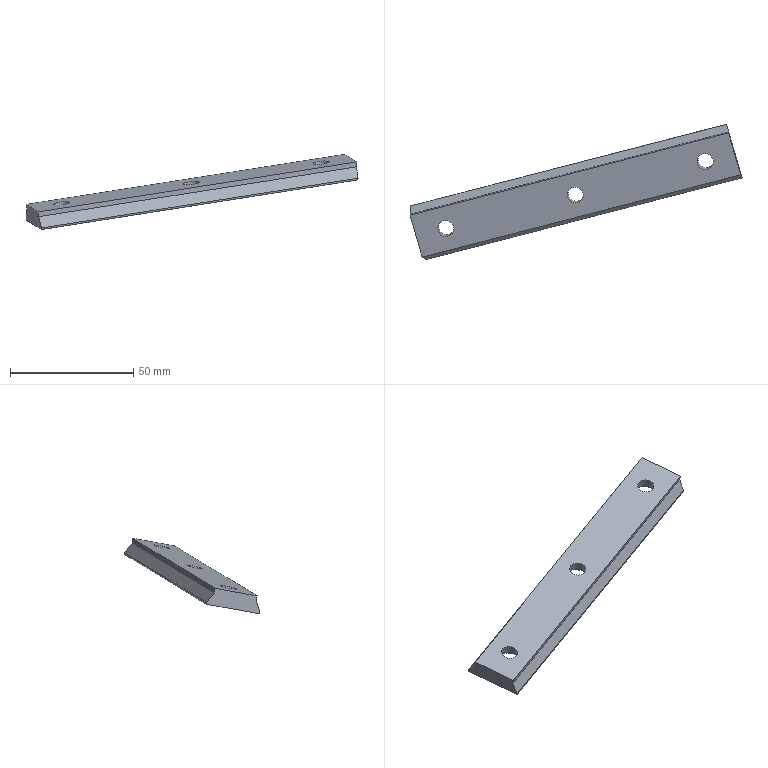Part | STEP file | 车灯-后视镜_id114_x_t | 1 solid | 19 faces | box 134.693 x 54.944 x 30.493 mm | volume 17624 mm3 | plane 8 | cylinder 8 | cone 3 | commonest cylinder face diameters 6.5 x3 12 x3 1 x2
STEP:
#1=CARTESIAN_POINT('',(43.374,63.133,39.053));
#2=VERTEX_POINT('',#1);
#3=CARTESIAN_POINT('',(43.332,63.478,37.067));
#4=VERTEX_POINT('',#3);
#5=CARTESIAN_POINT('',(43.54,61.75,47.027));
#6=DIRECTION('',(-0.02054,0.1709,-0.9851));
#7=VECTOR('',#6,1.);
#8=LINE('',#5,#7);
#9=EDGE_CURVE('',#2,#4,#8,.T.);
#10=ORIENTED_EDGE('',*,*,#9,.T.);
#11=CARTESIAN_POINT('',(43.909,61.886,32.43));
#12=VERTEX_POINT('',#11);
#13=CARTESIAN_POINT('',(42.508,65.752,43.692));
#14=DIRECTION('',(0.1169,-0.3225,-0.9393));
#15=VECTOR('',#14,1.);
#16=LINE('',#13,#15);
#17=EDGE_CURVE('',#4,#12,#16,.T.);
#18=ORIENTED_EDGE('',*,*,#17,.T.);
#19=CARTESIAN_POINT('',(43.776,62.425,31.759));
#20=VERTEX_POINT('',#19);
#21=CARTESIAN_POINT('',(43.787,62.339,32.255));
#22=DIRECTION('',(-0.9623,-0.2705,-0.02686));
#23=DIRECTION('',(-0.02054,0.1709,-0.9851));
#24=AXIS2_PLACEMENT_3D('',#21,#22,#23);
#25=ELLIPSE('',#24,0.504,0.5);
#26=EDGE_CURVE('',#20,#12,#25,.T.);
#27=ORIENTED_EDGE('',*,*,#26,.F.);
#28=CARTESIAN_POINT('',(37.813,83.27,35.499));
#29=VERTEX_POINT('',#28);
#30=CARTESIAN_POINT('',(36.98,86.182,36.022));
#31=DIRECTION('',(-0.271,0.9474,0.17));
#32=VECTOR('',#31,1.);
#33=LINE('',#30,#32);
#34=EDGE_CURVE('',#20,#29,#33,.T.);
#35=ORIENTED_EDGE('',*,*,#34,.T.);
#36=CARTESIAN_POINT('',(37.711,83.551,36.318));
#37=VERTEX_POINT('',#36);
#38=CARTESIAN_POINT('',(37.823,83.184,35.996));
#39=DIRECTION('',(-0.9623,-0.2705,-0.02686));
#40=DIRECTION('',(0.02054,-0.1709,0.9851));
#41=AXIS2_PLACEMENT_3D('',#38,#39,#40);
#42=ELLIPSE('',#41,0.504,0.5);
#43=EDGE_CURVE('',#37,#29,#42,.T.);
#44=ORIENTED_EDGE('',*,*,#43,.F.);
#45=CARTESIAN_POINT('',(38.464,80.495,40.121));
#46=VERTEX_POINT('',#45);
#47=CARTESIAN_POINT('',(39.547,76.099,45.591));
#48=DIRECTION('',(-0.1525,0.6191,-0.7704));
#49=VECTOR('',#48,1.);
#50=LINE('',#47,#49);
#51=EDGE_CURVE('',#46,#37,#50,.T.);
#52=ORIENTED_EDGE('',*,*,#51,.F.);
#53=CARTESIAN_POINT('',(38.505,80.151,42.106));
#54=VERTEX_POINT('',#53);
#55=CARTESIAN_POINT('',(38.673,78.758,50.135));
#56=DIRECTION('',(-0.02054,0.1709,-0.9851));
#57=VECTOR('',#56,1.);
#58=LINE('',#55,#57);
#59=EDGE_CURVE('',#54,#46,#58,.T.);
#60=ORIENTED_EDGE('',*,*,#59,.F.);
#61=CARTESIAN_POINT('',(37.125,84.976,42.972));
#62=DIRECTION('',(-0.271,0.9474,0.17));
#63=VECTOR('',#62,1.);
#64=LINE('',#61,#63);
#65=EDGE_CURVE('',#2,#54,#64,.T.);
#66=ORIENTED_EDGE('',*,*,#65,.F.);
#67=EDGE_LOOP('',(#10,#18,#27,#35,#44,#52,#60,#66));
#68=FACE_OUTER_BOUND('',#67,.T.);
#69=CARTESIAN_POINT('',(38.505,80.151,42.106));
#70=DIRECTION('',(0.9623,0.2705,0.02686));
#71=DIRECTION('',(-0.2706,0.9627,0.));
#72=AXIS2_PLACEMENT_3D('',#69,#70,#71);
#73=PLANE('',#72);
#74=ADVANCED_FACE('',(#68),#73,.T.);
#75=CARTESIAN_POINT('',(-84.613,29.308,11.621));
#76=VERTEX_POINT('',#75);
#77=CARTESIAN_POINT('',(-90.576,50.153,15.361));
#78=VERTEX_POINT('',#77);
#79=CARTESIAN_POINT('',(-90.029,48.239,15.018));
#80=DIRECTION('',(-0.271,0.9474,0.17));
#81=VECTOR('',#80,1.);
#82=LINE('',#79,#81);
#83=EDGE_CURVE('',#76,#78,#82,.T.);
#84=ORIENTED_EDGE('',*,*,#83,.F.);
#85=CARTESIAN_POINT('',(-84.571,28.745,12.277));
#86=VERTEX_POINT('',#85);
#87=CARTESIAN_POINT('',(-84.663,29.206,12.108));
#88=DIRECTION('',(-0.9573,-0.2469,-0.1502));
#89=DIRECTION('',(-0.2498,0.9683,0.));
#90=AXIS2_PLACEMENT_3D('',#87,#88,#89);
#91=CIRCLE('',#90,0.5);
#92=EDGE_CURVE('',#76,#86,#91,.T.);
#93=ORIENTED_EDGE('',*,*,#92,.T.);
#94=CARTESIAN_POINT('',(-85.662,30.205,16.834));
#95=VERTEX_POINT('',#94);
#96=CARTESIAN_POINT('',(-88.043,33.39,26.779));
#97=DIRECTION('',(0.2224,-0.2974,-0.9285));
#98=VECTOR('',#97,1.);
#99=LINE('',#96,#98);
#100=EDGE_CURVE('',#95,#86,#99,.T.);
#101=ORIENTED_EDGE('',*,*,#100,.F.);
#102=CARTESIAN_POINT('',(-85.862,29.798,18.782));
#103=VERTEX_POINT('',#102);
#104=CARTESIAN_POINT('',(-85.862,29.798,18.782));
#105=DIRECTION('',(0.1003,0.2035,-0.9739));
#106=VECTOR('',#105,1.);
#107=LINE('',#104,#106);
#108=EDGE_CURVE('',#103,#95,#107,.T.);
#109=ORIENTED_EDGE('',*,*,#108,.F.);
#110=CARTESIAN_POINT('',(-90.731,46.815,21.835));
#111=VERTEX_POINT('',#110);
#112=CARTESIAN_POINT('',(-90.731,46.815,21.835));
#113=DIRECTION('',(-0.271,0.9474,0.17));
#114=VECTOR('',#113,1.);
#115=LINE('',#112,#114);
#116=EDGE_CURVE('',#103,#111,#115,.T.);
#117=ORIENTED_EDGE('',*,*,#116,.T.);
#118=CARTESIAN_POINT('',(-90.53,47.222,19.887));
#119=VERTEX_POINT('',#118);
#120=CARTESIAN_POINT('',(-90.731,46.815,21.835));
#121=DIRECTION('',(0.1003,0.2035,-0.9739));
#122=VECTOR('',#121,1.);
#123=LINE('',#120,#122);
#124=EDGE_CURVE('',#111,#119,#123,.T.);
#125=ORIENTED_EDGE('',*,*,#124,.T.);
#126=CARTESIAN_POINT('',(-90.769,50.411,16.165));
#127=VERTEX_POINT('',#126);
#128=CARTESIAN_POINT('',(-90.446,46.096,21.201));
#129=DIRECTION('',(-0.04864,0.6498,-0.7585));
#130=VECTOR('',#129,1.);
#131=LINE('',#128,#130);
#132=EDGE_CURVE('',#119,#127,#131,.T.);
#133=ORIENTED_EDGE('',*,*,#132,.T.);
#134=CARTESIAN_POINT('',(-90.626,50.051,15.848));
#135=DIRECTION('',(-0.9573,-0.2469,-0.1502));
#136=DIRECTION('',(-0.2498,0.9683,0.));
#137=AXIS2_PLACEMENT_3D('',#134,#135,#136);
#138=CIRCLE('',#137,0.5);
#139=EDGE_CURVE('',#127,#78,#138,.T.);
#140=ORIENTED_EDGE('',*,*,#139,.T.);
#141=EDGE_LOOP('',(#84,#93,#101,#109,#117,#125,#133,#140));
#142=FACE_OUTER_BOUND('',#141,.T.);
#143=CARTESIAN_POINT('',(-90.731,46.815,21.835));
#144=DIRECTION('',(0.9573,0.2469,0.1502));
#145=DIRECTION('',(-0.2498,0.9683,0.));
#146=AXIS2_PLACEMENT_3D('',#143,#144,#145);
#147=PLANE('',#146);
#148=ADVANCED_FACE('',(#142),#147,.F.);
#149=CARTESIAN_POINT('',(-90.701,50.428,16.176));
#150=DIRECTION('',(-0.9573,-0.2469,-0.1502));
#151=VECTOR('',#150,1.);
#152=LINE('',#149,#151);
#153=EDGE_CURVE('',#37,#127,#152,.T.);
#154=ORIENTED_EDGE('',*,*,#153,.F.);
#155=ORIENTED_EDGE('',*,*,#43,.T.);
#156=CARTESIAN_POINT('',(100.957,99.558,45.404));
#157=DIRECTION('',(0.9573,0.2469,0.1502));
#158=VECTOR('',#157,1.);
#159=LINE('',#156,#158);
#160=EDGE_CURVE('',#78,#29,#159,.T.);
#161=ORIENTED_EDGE('',*,*,#160,.F.);
#162=ORIENTED_EDGE('',*,*,#139,.F.);
#163=EDGE_LOOP('',(#154,#155,#161,#162));
#164=FACE_OUTER_BOUND('',#163,.T.);
#165=CARTESIAN_POINT('',(100.839,99.438,45.88));
#166=DIRECTION('',(0.9573,0.2469,0.1502));
#167=DIRECTION('',(-0.2498,0.9683,0.));
#168=AXIS2_PLACEMENT_3D('',#165,#166,#167);
#169=CYLINDRICAL_SURFACE('',#168,0.5);
#170=ADVANCED_FACE('',(#164),#169,.T.);
#171=CARTESIAN_POINT('',(106.972,78.726,41.671));
#172=DIRECTION('',(-0.9573,-0.2469,-0.1502));
#173=VECTOR('',#172,1.);
#174=LINE('',#171,#173);
#175=EDGE_CURVE('',#20,#76,#174,.T.);
#176=ORIENTED_EDGE('',*,*,#175,.F.);
#177=ORIENTED_EDGE('',*,*,#26,.T.);
#178=CARTESIAN_POINT('',(106.473,78.023,42.243));
#179=DIRECTION('',(0.9573,0.2469,0.1502));
#180=VECTOR('',#179,1.);
#181=LINE('',#178,#180);
#182=EDGE_CURVE('',#86,#12,#181,.T.);
#183=ORIENTED_EDGE('',*,*,#182,.F.);
#184=ORIENTED_EDGE('',*,*,#92,.F.);
#185=EDGE_LOOP('',(#176,#177,#183,#184));
#186=FACE_OUTER_BOUND('',#185,.T.);
#187=CARTESIAN_POINT('',(106.922,78.624,42.158));
#188=DIRECTION('',(-0.9573,-0.2469,-0.1502));
#189=DIRECTION('',(0.2498,-0.9683,0.));
#190=AXIS2_PLACEMENT_3D('',#187,#188,#189);
#191=CYLINDRICAL_SURFACE('',#190,0.5);
#192=ADVANCED_FACE('',(#186),#191,.T.);
#193=CARTESIAN_POINT('',(28.976,65.375,38.038));
#194=VERTEX_POINT('',#193);
#195=CARTESIAN_POINT('',(28.976,68.556,38.703));
#196=DIRECTION('',(-0.1003,-0.2035,0.9739));
#197=DIRECTION('',(0.,-0.9789,-0.2045));
#198=AXIS2_PLACEMENT_3D('',#195,#196,#197);
#199=CIRCLE('',#198,3.25);
#200=EDGE_CURVE('',#194,#194,#199,.T.);
#201=ORIENTED_EDGE('',*,*,#200,.F.);
#202=EDGE_LOOP('',(#201));
#203=FACE_BOUND('',#202,.T.);
#204=CARTESIAN_POINT('',(-76.33,38.212,21.521));
#205=VERTEX_POINT('',#204);
#206=CARTESIAN_POINT('',(-76.33,41.393,22.185));
#207=DIRECTION('',(-0.1003,-0.2035,0.9739));
#208=DIRECTION('',(0.,-0.9789,-0.2045));
#209=AXIS2_PLACEMENT_3D('',#206,#207,#208);
#210=CIRCLE('',#209,3.25);
#211=EDGE_CURVE('',#205,#205,#210,.T.);
#212=ORIENTED_EDGE('',*,*,#211,.F.);
#213=EDGE_LOOP('',(#212));
#214=FACE_BOUND('',#213,.T.);
#215=CARTESIAN_POINT('',(-23.677,51.793,29.78));
#216=VERTEX_POINT('',#215);
#217=CARTESIAN_POINT('',(-23.677,54.975,30.444));
#218=DIRECTION('',(-0.1003,-0.2035,0.9739));
#219=DIRECTION('',(0.,-0.9789,-0.2045));
#220=AXIS2_PLACEMENT_3D('',#217,#218,#219);
#221=CIRCLE('',#220,3.25);
#222=EDGE_CURVE('',#216,#216,#221,.T.);
#223=ORIENTED_EDGE('',*,*,#222,.F.);
#224=EDGE_LOOP('',(#223));
#225=FACE_BOUND('',#224,.T.);
#226=CARTESIAN_POINT('',(105.181,79.076,48.747));
#227=DIRECTION('',(-0.9573,-0.2469,-0.1502));
#228=VECTOR('',#227,1.);
#229=LINE('',#226,#228);
#230=EDGE_CURVE('',#2,#103,#229,.T.);
#231=ORIENTED_EDGE('',*,*,#230,.F.);
#232=ORIENTED_EDGE('',*,*,#65,.T.);
#233=CARTESIAN_POINT('',(100.735,96.202,51.867));
#234=DIRECTION('',(-0.9573,-0.2469,-0.1502));
#235=VECTOR('',#234,1.);
#236=LINE('',#233,#235);
#237=EDGE_CURVE('',#54,#111,#236,.T.);
#238=ORIENTED_EDGE('',*,*,#237,.T.);
#239=ORIENTED_EDGE('',*,*,#116,.F.);
#240=EDGE_LOOP('',(#231,#232,#238,#239));
#241=FACE_BOUND('',#240,.T.);
#242=CARTESIAN_POINT('',(99.474,101.059,52.752));
#243=DIRECTION('',(-0.1003,-0.2035,0.9739));
#244=DIRECTION('',(0.,-0.9789,-0.2045));
#245=AXIS2_PLACEMENT_3D('',#242,#243,#244);
#246=PLANE('',#245);
#247=ADVANCED_FACE('',(#203,#214,#225,#241),#246,.T.);
#248=ORIENTED_EDGE('',*,*,#9,.F.);
#249=ORIENTED_EDGE('',*,*,#230,.T.);
#250=ORIENTED_EDGE('',*,*,#108,.T.);
#251=CARTESIAN_POINT('',(105.382,79.483,46.8));
#252=DIRECTION('',(-0.9573,-0.2469,-0.1502));
#253=VECTOR('',#252,1.);
#254=LINE('',#251,#253);
#255=EDGE_CURVE('',#4,#95,#254,.T.);
#256=ORIENTED_EDGE('',*,*,#255,.F.);
#257=EDGE_LOOP('',(#248,#249,#250,#256));
#258=FACE_OUTER_BOUND('',#257,.T.);
#259=CARTESIAN_POINT('',(105.181,79.076,48.747));
#260=DIRECTION('',(-0.271,0.9474,0.17));
#261=DIRECTION('',(-0.9614,-0.2751,0.));
#262=AXIS2_PLACEMENT_3D('',#259,#260,#261);
#263=PLANE('',#262);
#264=ADVANCED_FACE('',(#258),#263,.F.);
#265=ORIENTED_EDGE('',*,*,#17,.F.);
#266=ORIENTED_EDGE('',*,*,#255,.T.);
#267=ORIENTED_EDGE('',*,*,#100,.T.);
#268=ORIENTED_EDGE('',*,*,#182,.T.);
#269=EDGE_LOOP('',(#265,#266,#267,#268));
#270=FACE_OUTER_BOUND('',#269,.T.);
#271=CARTESIAN_POINT('',(105.382,79.483,46.8));
#272=DIRECTION('',(-0.1846,0.9223,-0.3396));
#273=DIRECTION('',(0.,0.3456,0.9384));
#274=AXIS2_PLACEMENT_3D('',#271,#272,#273);
#275=PLANE('',#274);
#276=ADVANCED_FACE('',(#270),#275,.F.);
#277=CARTESIAN_POINT('',(31.304,64.296,30.865));
#278=VERTEX_POINT('',#277);
#279=CARTESIAN_POINT('',(29.678,69.98,31.885));
#280=DIRECTION('',(-0.1003,-0.2035,0.9739));
#281=DIRECTION('',(0.271,-0.9474,-0.17));
#282=AXIS2_PLACEMENT_3D('',#279,#280,#281);
#283=CIRCLE('',#282,6.);
#284=EDGE_CURVE('',#278,#278,#283,.T.);
#285=ORIENTED_EDGE('',*,*,#284,.T.);
#286=EDGE_LOOP('',(#285));
#287=FACE_BOUND('',#286,.T.);
#288=CARTESIAN_POINT('',(-74.002,37.133,14.348));
#289=VERTEX_POINT('',#288);
#290=CARTESIAN_POINT('',(-75.628,42.817,15.368));
#291=DIRECTION('',(-0.1003,-0.2035,0.9739));
#292=DIRECTION('',(0.271,-0.9474,-0.17));
#293=AXIS2_PLACEMENT_3D('',#290,#291,#292);
#294=CIRCLE('',#293,6.);
#295=EDGE_CURVE('',#289,#289,#294,.T.);
#296=ORIENTED_EDGE('',*,*,#295,.T.);
#297=EDGE_LOOP('',(#296));
#298=FACE_BOUND('',#297,.T.);
#299=CARTESIAN_POINT('',(-21.349,50.714,22.607));
#300=VERTEX_POINT('',#299);
#301=CARTESIAN_POINT('',(-22.975,56.399,23.627));
#302=DIRECTION('',(-0.1003,-0.2035,0.9739));
#303=DIRECTION('',(0.271,-0.9474,-0.17));
#304=AXIS2_PLACEMENT_3D('',#301,#302,#303);
#305=CIRCLE('',#304,6.);
#306=EDGE_CURVE('',#300,#300,#305,.T.);
#307=ORIENTED_EDGE('',*,*,#306,.T.);
#308=EDGE_LOOP('',(#307));
#309=FACE_BOUND('',#308,.T.);
#310=ORIENTED_EDGE('',*,*,#34,.F.);
#311=ORIENTED_EDGE('',*,*,#175,.T.);
#312=ORIENTED_EDGE('',*,*,#83,.T.);
#313=ORIENTED_EDGE('',*,*,#160,.T.);
#314=EDGE_LOOP('',(#310,#311,#312,#313));
#315=FACE_BOUND('',#314,.T.);
#316=CARTESIAN_POINT('',(100.176,102.483,45.934));
#317=DIRECTION('',(-0.1003,-0.2035,0.9739));
#318=DIRECTION('',(0.,-0.9789,-0.2045));
#319=AXIS2_PLACEMENT_3D('',#316,#317,#318);
#320=PLANE('',#319);
#321=ADVANCED_FACE('',(#287,#298,#309,#315),#320,.F.);
#322=CARTESIAN_POINT('',(100.935,96.609,49.919));
#323=DIRECTION('',(-0.9573,-0.2469,-0.1502));
#324=VECTOR('',#323,1.);
#325=LINE('',#322,#324);
#326=EDGE_CURVE('',#46,#119,#325,.T.);
#327=ORIENTED_EDGE('',*,*,#326,.F.);
#328=ORIENTED_EDGE('',*,*,#51,.T.);
#329=ORIENTED_EDGE('',*,*,#153,.T.);
#330=ORIENTED_EDGE('',*,*,#132,.F.);
#331=EDGE_LOOP('',(#327,#328,#329,#330));
#332=FACE_OUTER_BOUND('',#331,.T.);
#333=CARTESIAN_POINT('',(100.935,96.609,49.919));
#334=DIRECTION('',(-0.2849,0.7189,0.6341));
#335=DIRECTION('',(0.,-0.6615,0.7499));
#336=AXIS2_PLACEMENT_3D('',#333,#334,#335);
#337=PLANE('',#336);
#338=ADVANCED_FACE('',(#332),#337,.T.);
#339=ORIENTED_EDGE('',*,*,#237,.F.);
#340=ORIENTED_EDGE('',*,*,#59,.T.);
#341=ORIENTED_EDGE('',*,*,#326,.T.);
#342=ORIENTED_EDGE('',*,*,#124,.F.);
#343=EDGE_LOOP('',(#339,#340,#341,#342));
#344=FACE_OUTER_BOUND('',#343,.T.);
#345=CARTESIAN_POINT('',(100.735,96.202,51.867));
#346=DIRECTION('',(-0.271,0.9474,0.17));
#347=DIRECTION('',(-0.9614,-0.2751,0.));
#348=AXIS2_PLACEMENT_3D('',#345,#346,#347);
#349=PLANE('',#348);
#350=ADVANCED_FACE('',(#344),#349,.T.);
#351=CARTESIAN_POINT('',(-21.429,50.551,23.386));
#352=VERTEX_POINT('',#351);
#353=CARTESIAN_POINT('',(-23.055,56.236,24.406));
#354=DIRECTION('',(-0.1003,-0.2035,0.9739));
#355=DIRECTION('',(0.271,-0.9474,-0.17));
#356=AXIS2_PLACEMENT_3D('',#353,#354,#355);
#357=CIRCLE('',#356,6.);
#358=EDGE_CURVE('',#352,#352,#357,.T.);
#359=ORIENTED_EDGE('',*,*,#358,.T.);
#360=EDGE_LOOP('',(#359));
#361=FACE_BOUND('',#360,.T.);
#362=ORIENTED_EDGE('',*,*,#306,.F.);
#363=EDGE_LOOP('',(#362));
#364=FACE_BOUND('',#363,.T.);
#365=CARTESIAN_POINT('',(-23.025,56.297,24.114));
#366=DIRECTION('',(-0.1003,-0.2035,0.9739));
#367=DIRECTION('',(-0.271,0.9474,0.17));
#368=AXIS2_PLACEMENT_3D('',#365,#366,#367);
#369=CYLINDRICAL_SURFACE('',#368,6.);
#370=ADVANCED_FACE('',(#361,#364),#369,.F.);
#371=CARTESIAN_POINT('',(-22.45,52.597,26.532));
#372=VERTEX_POINT('',#371);
#373=CARTESIAN_POINT('',(-23.331,55.676,27.084));
#374=DIRECTION('',(-0.1003,-0.2035,0.9739));
#375=DIRECTION('',(0.271,-0.9474,-0.17));
#376=AXIS2_PLACEMENT_3D('',#373,#374,#375);
#377=CIRCLE('',#376,3.25);
#378=EDGE_CURVE('',#372,#372,#377,.T.);
#379=ORIENTED_EDGE('',*,*,#378,.T.);
#380=EDGE_LOOP('',(#379));
#381=FACE_BOUND('',#380,.T.);
#382=ORIENTED_EDGE('',*,*,#358,.F.);
#383=EDGE_LOOP('',(#382));
#384=FACE_BOUND('',#383,.T.);
#385=CARTESIAN_POINT('',(-23.055,56.236,24.406));
#386=DIRECTION('',(0.1003,0.2035,-0.9739));
#387=DIRECTION('',(-0.271,0.9474,0.17));
#388=AXIS2_PLACEMENT_3D('',#385,#386,#387);
#389=CONICAL_SURFACE('',#388,6.,45.);
#390=ADVANCED_FACE('',(#381,#384),#389,.F.);
#391=ORIENTED_EDGE('',*,*,#222,.T.);
#392=EDGE_LOOP('',(#391));
#393=FACE_BOUND('',#392,.T.);
#394=ORIENTED_EDGE('',*,*,#378,.F.);
#395=EDGE_LOOP('',(#394));
#396=FACE_BOUND('',#395,.T.);
#397=CARTESIAN_POINT('',(-23.356,55.626,27.328));
#398=DIRECTION('',(-0.1003,-0.2035,0.9739));
#399=DIRECTION('',(-0.271,0.9474,0.17));
#400=AXIS2_PLACEMENT_3D('',#397,#398,#399);
#401=CYLINDRICAL_SURFACE('',#400,3.25);
#402=ADVANCED_FACE('',(#393,#396),#401,.F.);
#403=CARTESIAN_POINT('',(-74.082,36.97,15.127));
#404=VERTEX_POINT('',#403);
#405=CARTESIAN_POINT('',(-75.708,42.655,16.147));
#406=DIRECTION('',(-0.1003,-0.2035,0.9739));
#407=DIRECTION('',(0.271,-0.9474,-0.17));
#408=AXIS2_PLACEMENT_3D('',#405,#406,#407);
#409=CIRCLE('',#408,6.);
#410=EDGE_CURVE('',#404,#404,#409,.T.);
#411=ORIENTED_EDGE('',*,*,#410,.T.);
#412=EDGE_LOOP('',(#411));
#413=FACE_BOUND('',#412,.T.);
#414=ORIENTED_EDGE('',*,*,#295,.F.);
#415=EDGE_LOOP('',(#414));
#416=FACE_BOUND('',#415,.T.);
#417=CARTESIAN_POINT('',(-75.678,42.716,15.855));
#418=DIRECTION('',(-0.1003,-0.2035,0.9739));
#419=DIRECTION('',(-0.271,0.9474,0.17));
#420=AXIS2_PLACEMENT_3D('',#417,#418,#419);
#421=CYLINDRICAL_SURFACE('',#420,6.);
#422=ADVANCED_FACE('',(#413,#416),#421,.F.);
#423=CARTESIAN_POINT('',(-75.103,39.016,18.273));
#424=VERTEX_POINT('',#423);
#425=CARTESIAN_POINT('',(-75.984,42.095,18.825));
#426=DIRECTION('',(-0.1003,-0.2035,0.9739));
#427=DIRECTION('',(0.271,-0.9474,-0.17));
#428=AXIS2_PLACEMENT_3D('',#425,#426,#427);
#429=CIRCLE('',#428,3.25);
#430=EDGE_CURVE('',#424,#424,#429,.T.);
#431=ORIENTED_EDGE('',*,*,#430,.T.);
#432=EDGE_LOOP('',(#431));
#433=FACE_BOUND('',#432,.T.);
#434=ORIENTED_EDGE('',*,*,#410,.F.);
#435=EDGE_LOOP('',(#434));
#436=FACE_BOUND('',#435,.T.);
#437=CARTESIAN_POINT('',(-75.708,42.655,16.147));
#438=DIRECTION('',(0.1003,0.2035,-0.9739));
#439=DIRECTION('',(-0.271,0.9474,0.17));
#440=AXIS2_PLACEMENT_3D('',#437,#438,#439);
#441=CONICAL_SURFACE('',#440,6.,45.);
#442=ADVANCED_FACE('',(#433,#436),#441,.F.);
#443=ORIENTED_EDGE('',*,*,#211,.T.);
#444=EDGE_LOOP('',(#443));
#445=FACE_BOUND('',#444,.T.);
#446=ORIENTED_EDGE('',*,*,#430,.F.);
#447=EDGE_LOOP('',(#446));
#448=FACE_BOUND('',#447,.T.);
#449=CARTESIAN_POINT('',(-76.009,42.044,19.069));
#450=DIRECTION('',(-0.1003,-0.2035,0.9739));
#451=DIRECTION('',(-0.271,0.9474,0.17));
#452=AXIS2_PLACEMENT_3D('',#449,#450,#451);
#453=CYLINDRICAL_SURFACE('',#452,3.25);
#454=ADVANCED_FACE('',(#445,#448),#453,.F.);
#455=CARTESIAN_POINT('',(31.224,64.133,31.645));
#456=VERTEX_POINT('',#455);
#457=CARTESIAN_POINT('',(29.598,69.817,32.665));
#458=DIRECTION('',(-0.1003,-0.2035,0.9739));
#459=DIRECTION('',(0.271,-0.9474,-0.17));
#460=AXIS2_PLACEMENT_3D('',#457,#458,#459);
#461=CIRCLE('',#460,6.);
#462=EDGE_CURVE('',#456,#456,#461,.T.);
#463=ORIENTED_EDGE('',*,*,#462,.T.);
#464=EDGE_LOOP('',(#463));
#465=FACE_BOUND('',#464,.T.);
#466=ORIENTED_EDGE('',*,*,#284,.F.);
#467=EDGE_LOOP('',(#466));
#468=FACE_BOUND('',#467,.T.);
#469=CARTESIAN_POINT('',(29.628,69.878,32.372));
#470=DIRECTION('',(-0.1003,-0.2035,0.9739));
#471=DIRECTION('',(-0.271,0.9474,0.17));
#472=AXIS2_PLACEMENT_3D('',#469,#470,#471);
#473=CYLINDRICAL_SURFACE('',#472,6.);
#474=ADVANCED_FACE('',(#465,#468),#473,.F.);
#475=CARTESIAN_POINT('',(30.203,66.179,34.79));
#476=VERTEX_POINT('',#475);
#477=CARTESIAN_POINT('',(29.322,69.258,35.343));
#478=DIRECTION('',(-0.1003,-0.2035,0.9739));
#479=DIRECTION('',(0.271,-0.9474,-0.17));
#480=AXIS2_PLACEMENT_3D('',#477,#478,#479);
#481=CIRCLE('',#480,3.25);
#482=EDGE_CURVE('',#476,#476,#481,.T.);
#483=ORIENTED_EDGE('',*,*,#482,.T.);
#484=EDGE_LOOP('',(#483));
#485=FACE_BOUND('',#484,.T.);
#486=ORIENTED_EDGE('',*,*,#462,.F.);
#487=EDGE_LOOP('',(#486));
#488=FACE_BOUND('',#487,.T.);
#489=CARTESIAN_POINT('',(29.598,69.817,32.665));
#490=DIRECTION('',(0.1003,0.2035,-0.9739));
#491=DIRECTION('',(-0.271,0.9474,0.17));
#492=AXIS2_PLACEMENT_3D('',#489,#490,#491);
#493=CONICAL_SURFACE('',#492,6.,45.);
#494=ADVANCED_FACE('',(#485,#488),#493,.F.);
#495=ORIENTED_EDGE('',*,*,#200,.T.);
#496=EDGE_LOOP('',(#495));
#497=FACE_BOUND('',#496,.T.);
#498=ORIENTED_EDGE('',*,*,#482,.F.);
#499=EDGE_LOOP('',(#498));
#500=FACE_BOUND('',#499,.T.);
#501=CARTESIAN_POINT('',(29.297,69.207,35.586));
#502=DIRECTION('',(-0.1003,-0.2035,0.9739));
#503=DIRECTION('',(-0.271,0.9474,0.17));
#504=AXIS2_PLACEMENT_3D('',#501,#502,#503);
#505=CYLINDRICAL_SURFACE('',#504,3.25);
#506=ADVANCED_FACE('',(#497,#500),#505,.F.);
#507=CLOSED_SHELL('',(#74,#148,#170,#192,#247,#264,#276,#321,#338,#350,#370,#390,#402,#422,#442,#454,#474,#494,#506));
#508=MANIFOLD_SOLID_BREP('',#507);
#509=(LENGTH_UNIT()NAMED_UNIT(*)SI_UNIT(.MILLI.,.METRE.));
#510=UNCERTAINTY_MEASURE_WITH_UNIT(LENGTH_MEASURE(0.00002),#509,'','');
#511=(NAMED_UNIT(*)PLANE_ANGLE_UNIT()SI_UNIT($,.RADIAN.));
#512=PLANE_ANGLE_MEASURE_WITH_UNIT(PLANE_ANGLE_MEASURE(0.01745),#511);
#513=DIMENSIONAL_EXPONENTS(0.,0.,0.,0.,0.,0.,0.);
#514=(CONVERSION_BASED_UNIT('DEGREE',#512)NAMED_UNIT(#513)PLANE_ANGLE_UNIT());
#515=(NAMED_UNIT(*)SI_UNIT($,.STERADIAN.)SOLID_ANGLE_UNIT());
#516=(GEOMETRIC_REPRESENTATION_CONTEXT(3)GLOBAL_UNCERTAINTY_ASSIGNED_CONTEXT((#510))GLOBAL_UNIT_ASSIGNED_CONTEXT((#509,#514,#515))REPRESENTATION_CONTEXT('',''));
#517=ADVANCED_BREP_SHAPE_REPRESENTATION('',(#508),#516);